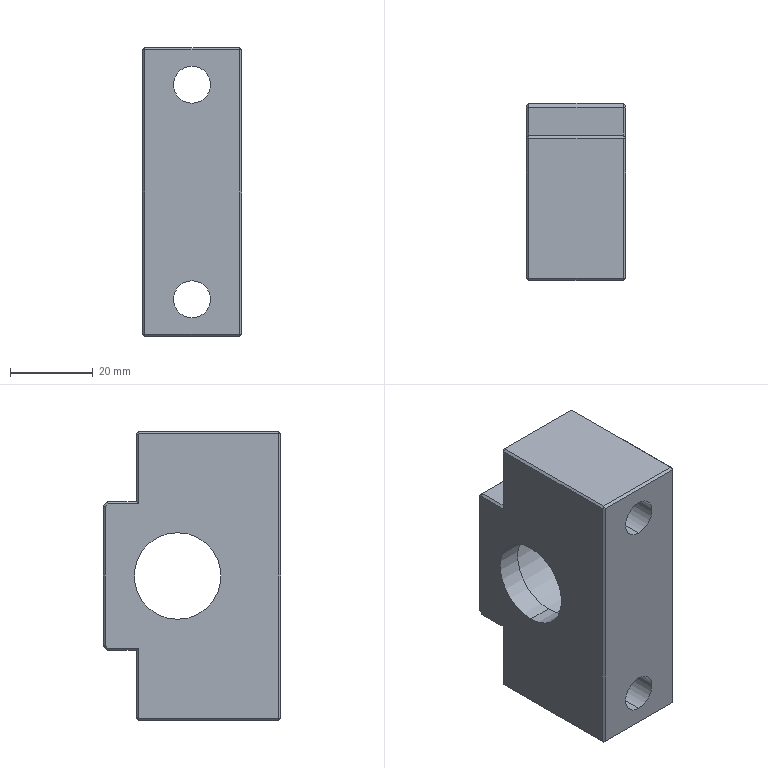Part | SolidWorks | features BaseBody 1 | 1 solid | 83 faces | box 24 x 43 x 70 mm | volume 47260 mm3 | plane 47 | cylinder 20 | cone 16 | commonest cylinder face diameters 3.242 x8 9 x4 14 x4 21 x2 26 x2